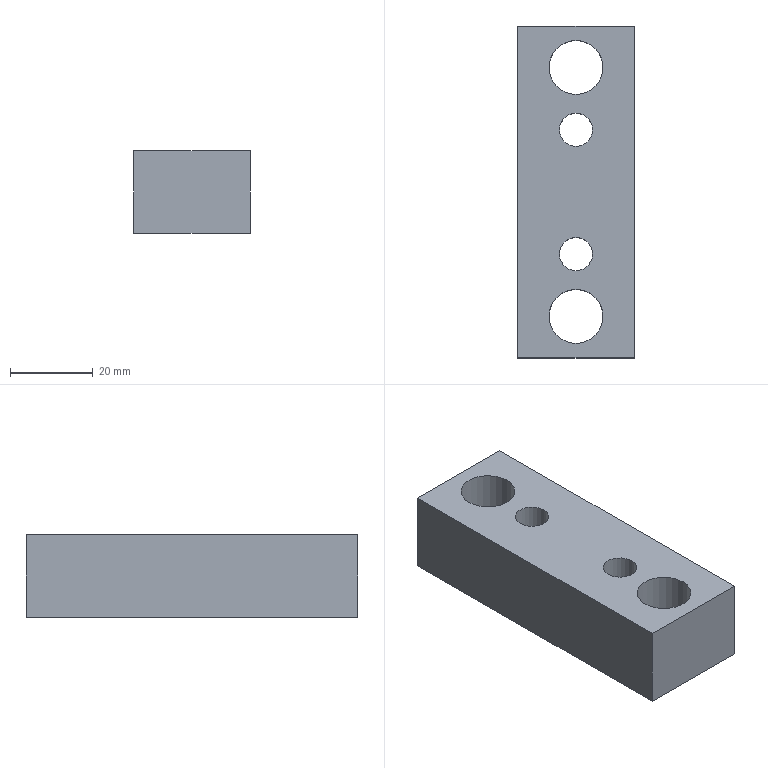Part | NX | features solid 2 | 1 solid | 10 faces | box 28 x 80 x 20 mm | volume 37480 mm3 | plane 6 | cylinder 4 | commonest cylinder face diameters 8 x2 13 x2
STEP:
#1=CARTESIAN_POINT('',(-1190.,-545.,-125.));
#2=VERTEX_POINT('',#1);
#3=CARTESIAN_POINT('',(-1190.,-625.,-125.));
#4=VERTEX_POINT('',#3);
#5=CARTESIAN_POINT('',(-1190.,-545.,-125.));
#6=DIRECTION('',(0.,-1.,0.));
#7=VECTOR('',#6,1000.);
#8=LINE('',#5,#7);
#9=EDGE_CURVE('',#2,#4,#8,.T.);
#10=ORIENTED_EDGE('',*,*,#9,.F.);
#11=CARTESIAN_POINT('',(-1190.,-545.,-105.));
#12=VERTEX_POINT('',#11);
#13=CARTESIAN_POINT('',(-1190.,-545.,-105.));
#14=DIRECTION('',(0.,0.,-1.));
#15=VECTOR('',#14,1000.);
#16=LINE('',#13,#15);
#17=EDGE_CURVE('',#12,#2,#16,.T.);
#18=ORIENTED_EDGE('',*,*,#17,.F.);
#19=CARTESIAN_POINT('',(-1190.,-625.,-105.));
#20=VERTEX_POINT('',#19);
#21=CARTESIAN_POINT('',(-1190.,-545.,-105.));
#22=DIRECTION('',(0.,-1.,0.));
#23=VECTOR('',#22,1000.);
#24=LINE('',#21,#23);
#25=EDGE_CURVE('',#12,#20,#24,.T.);
#26=ORIENTED_EDGE('',*,*,#25,.T.);
#27=CARTESIAN_POINT('',(-1190.,-625.,-105.));
#28=DIRECTION('',(0.,0.,-1.));
#29=VECTOR('',#28,1000.);
#30=LINE('',#27,#29);
#31=EDGE_CURVE('',#20,#4,#30,.T.);
#32=ORIENTED_EDGE('',*,*,#31,.T.);
#33=EDGE_LOOP('',(#10,#18,#26,#32));
#34=FACE_BOUND('',#33,.T.);
#35=CARTESIAN_POINT('',(-1190.,-545.,-105.));
#36=DIRECTION('',(1.,0.,0.));
#37=DIRECTION('',(0.,1.,0.));
#38=AXIS2_PLACEMENT_3D('',#35,#36,#37);
#39=PLANE('',#38);
#40=ADVANCED_FACE('',(#34),#39,.T.);
#41=CARTESIAN_POINT('',(-1218.,-625.,-125.));
#42=VERTEX_POINT('',#41);
#43=CARTESIAN_POINT('',(-1190.,-625.,-125.));
#44=DIRECTION('',(-1.,0.,0.));
#45=VECTOR('',#44,1000.);
#46=LINE('',#43,#45);
#47=EDGE_CURVE('',#4,#42,#46,.T.);
#48=ORIENTED_EDGE('',*,*,#47,.F.);
#49=ORIENTED_EDGE('',*,*,#31,.F.);
#50=CARTESIAN_POINT('',(-1218.,-625.,-105.));
#51=VERTEX_POINT('',#50);
#52=CARTESIAN_POINT('',(-1190.,-625.,-105.));
#53=DIRECTION('',(-1.,0.,0.));
#54=VECTOR('',#53,1000.);
#55=LINE('',#52,#54);
#56=EDGE_CURVE('',#20,#51,#55,.T.);
#57=ORIENTED_EDGE('',*,*,#56,.T.);
#58=CARTESIAN_POINT('',(-1218.,-625.,-105.));
#59=DIRECTION('',(0.,0.,-1.));
#60=VECTOR('',#59,1000.);
#61=LINE('',#58,#60);
#62=EDGE_CURVE('',#51,#42,#61,.T.);
#63=ORIENTED_EDGE('',*,*,#62,.T.);
#64=EDGE_LOOP('',(#48,#49,#57,#63));
#65=FACE_BOUND('',#64,.T.);
#66=CARTESIAN_POINT('',(-1190.,-625.,-105.));
#67=DIRECTION('',(0.,-1.,0.));
#68=DIRECTION('',(0.,0.,1.));
#69=AXIS2_PLACEMENT_3D('',#66,#67,#68);
#70=PLANE('',#69);
#71=ADVANCED_FACE('',(#65),#70,.T.);
#72=CARTESIAN_POINT('',(-1218.,-545.,-125.));
#73=VERTEX_POINT('',#72);
#74=CARTESIAN_POINT('',(-1218.,-625.,-125.));
#75=DIRECTION('',(0.,1.,0.));
#76=VECTOR('',#75,1000.);
#77=LINE('',#74,#76);
#78=EDGE_CURVE('',#42,#73,#77,.T.);
#79=ORIENTED_EDGE('',*,*,#78,.F.);
#80=ORIENTED_EDGE('',*,*,#62,.F.);
#81=CARTESIAN_POINT('',(-1218.,-545.,-105.));
#82=VERTEX_POINT('',#81);
#83=CARTESIAN_POINT('',(-1218.,-625.,-105.));
#84=DIRECTION('',(0.,1.,0.));
#85=VECTOR('',#84,1000.);
#86=LINE('',#83,#85);
#87=EDGE_CURVE('',#51,#82,#86,.T.);
#88=ORIENTED_EDGE('',*,*,#87,.T.);
#89=CARTESIAN_POINT('',(-1218.,-545.,-105.));
#90=DIRECTION('',(0.,0.,-1.));
#91=VECTOR('',#90,1000.);
#92=LINE('',#89,#91);
#93=EDGE_CURVE('',#82,#73,#92,.T.);
#94=ORIENTED_EDGE('',*,*,#93,.T.);
#95=EDGE_LOOP('',(#79,#80,#88,#94));
#96=FACE_BOUND('',#95,.T.);
#97=CARTESIAN_POINT('',(-1218.,-625.,-105.));
#98=DIRECTION('',(-1.,0.,0.));
#99=DIRECTION('',(0.,-1.,0.));
#100=AXIS2_PLACEMENT_3D('',#97,#98,#99);
#101=PLANE('',#100);
#102=ADVANCED_FACE('',(#96),#101,.T.);
#103=CARTESIAN_POINT('',(-1208.,-600.,-105.));
#104=VERTEX_POINT('',#103);
#105=CARTESIAN_POINT('',(-1204.,-600.,-105.));
#106=DIRECTION('',(0.,0.,1.));
#107=DIRECTION('',(-1.,0.,0.));
#108=AXIS2_PLACEMENT_3D('',#105,#106,#107);
#109=CIRCLE('',#108,4.);
#110=EDGE_CURVE('',#104,#104,#109,.T.);
#111=ORIENTED_EDGE('',*,*,#110,.T.);
#112=EDGE_LOOP('',(#111));
#113=FACE_BOUND('',#112,.T.);
#114=CARTESIAN_POINT('',(-1208.,-600.,-125.));
#115=VERTEX_POINT('',#114);
#116=CARTESIAN_POINT('',(-1204.,-600.,-125.));
#117=DIRECTION('',(0.,0.,1.));
#118=DIRECTION('',(-1.,0.,0.));
#119=AXIS2_PLACEMENT_3D('',#116,#117,#118);
#120=CIRCLE('',#119,4.);
#121=EDGE_CURVE('',#115,#115,#120,.T.);
#122=ORIENTED_EDGE('',*,*,#121,.F.);
#123=EDGE_LOOP('',(#122));
#124=FACE_BOUND('',#123,.T.);
#125=CARTESIAN_POINT('',(-1204.,-600.,-105.));
#126=DIRECTION('',(0.,0.,-1.));
#127=DIRECTION('',(1.,0.,0.));
#128=AXIS2_PLACEMENT_3D('',#125,#126,#127);
#129=CYLINDRICAL_SURFACE('',#128,4.);
#130=ADVANCED_FACE('',(#113,#124),#129,.F.);
#131=CARTESIAN_POINT('',(-1218.,-545.,-125.));
#132=DIRECTION('',(1.,0.,0.));
#133=VECTOR('',#132,1000.);
#134=LINE('',#131,#133);
#135=EDGE_CURVE('',#73,#2,#134,.T.);
#136=ORIENTED_EDGE('',*,*,#135,.F.);
#137=ORIENTED_EDGE('',*,*,#93,.F.);
#138=CARTESIAN_POINT('',(-1218.,-545.,-105.));
#139=DIRECTION('',(1.,0.,0.));
#140=VECTOR('',#139,1000.);
#141=LINE('',#138,#140);
#142=EDGE_CURVE('',#82,#12,#141,.T.);
#143=ORIENTED_EDGE('',*,*,#142,.T.);
#144=ORIENTED_EDGE('',*,*,#17,.T.);
#145=EDGE_LOOP('',(#136,#137,#143,#144));
#146=FACE_BOUND('',#145,.T.);
#147=CARTESIAN_POINT('',(-1218.,-545.,-105.));
#148=DIRECTION('',(0.,1.,0.));
#149=DIRECTION('',(-1.,0.,0.));
#150=AXIS2_PLACEMENT_3D('',#147,#148,#149);
#151=PLANE('',#150);
#152=ADVANCED_FACE('',(#146),#151,.T.);
#153=CARTESIAN_POINT('',(-1210.5,-615.,-105.));
#154=VERTEX_POINT('',#153);
#155=CARTESIAN_POINT('',(-1204.,-615.,-105.));
#156=DIRECTION('',(0.,0.,1.));
#157=DIRECTION('',(-1.,0.,0.));
#158=AXIS2_PLACEMENT_3D('',#155,#156,#157);
#159=CIRCLE('',#158,6.5);
#160=EDGE_CURVE('',#154,#154,#159,.T.);
#161=ORIENTED_EDGE('',*,*,#160,.T.);
#162=EDGE_LOOP('',(#161));
#163=FACE_BOUND('',#162,.T.);
#164=CARTESIAN_POINT('',(-1210.5,-615.,-125.));
#165=VERTEX_POINT('',#164);
#166=CARTESIAN_POINT('',(-1204.,-615.,-125.));
#167=DIRECTION('',(0.,0.,1.));
#168=DIRECTION('',(-1.,0.,0.));
#169=AXIS2_PLACEMENT_3D('',#166,#167,#168);
#170=CIRCLE('',#169,6.5);
#171=EDGE_CURVE('',#165,#165,#170,.T.);
#172=ORIENTED_EDGE('',*,*,#171,.F.);
#173=EDGE_LOOP('',(#172));
#174=FACE_BOUND('',#173,.T.);
#175=CARTESIAN_POINT('',(-1204.,-615.,-105.));
#176=DIRECTION('',(0.,0.,-1.));
#177=DIRECTION('',(1.,0.,0.));
#178=AXIS2_PLACEMENT_3D('',#175,#176,#177);
#179=CYLINDRICAL_SURFACE('',#178,6.5);
#180=ADVANCED_FACE('',(#163,#174),#179,.F.);
#181=CARTESIAN_POINT('',(-1208.,-570.,-105.));
#182=VERTEX_POINT('',#181);
#183=CARTESIAN_POINT('',(-1204.,-570.,-105.));
#184=DIRECTION('',(0.,0.,1.));
#185=DIRECTION('',(-1.,0.,0.));
#186=AXIS2_PLACEMENT_3D('',#183,#184,#185);
#187=CIRCLE('',#186,4.);
#188=EDGE_CURVE('',#182,#182,#187,.T.);
#189=ORIENTED_EDGE('',*,*,#188,.T.);
#190=EDGE_LOOP('',(#189));
#191=FACE_BOUND('',#190,.T.);
#192=CARTESIAN_POINT('',(-1208.,-570.,-125.));
#193=VERTEX_POINT('',#192);
#194=CARTESIAN_POINT('',(-1204.,-570.,-125.));
#195=DIRECTION('',(0.,0.,1.));
#196=DIRECTION('',(-1.,0.,0.));
#197=AXIS2_PLACEMENT_3D('',#194,#195,#196);
#198=CIRCLE('',#197,4.);
#199=EDGE_CURVE('',#193,#193,#198,.T.);
#200=ORIENTED_EDGE('',*,*,#199,.F.);
#201=EDGE_LOOP('',(#200));
#202=FACE_BOUND('',#201,.T.);
#203=CARTESIAN_POINT('',(-1204.,-570.,-105.));
#204=DIRECTION('',(0.,0.,-1.));
#205=DIRECTION('',(1.,0.,0.));
#206=AXIS2_PLACEMENT_3D('',#203,#204,#205);
#207=CYLINDRICAL_SURFACE('',#206,4.);
#208=ADVANCED_FACE('',(#191,#202),#207,.F.);
#209=CARTESIAN_POINT('',(-1210.5,-555.,-105.));
#210=VERTEX_POINT('',#209);
#211=CARTESIAN_POINT('',(-1204.,-555.,-105.));
#212=DIRECTION('',(0.,0.,1.));
#213=DIRECTION('',(-1.,0.,0.));
#214=AXIS2_PLACEMENT_3D('',#211,#212,#213);
#215=CIRCLE('',#214,6.5);
#216=EDGE_CURVE('',#210,#210,#215,.T.);
#217=ORIENTED_EDGE('',*,*,#216,.T.);
#218=EDGE_LOOP('',(#217));
#219=FACE_BOUND('',#218,.T.);
#220=CARTESIAN_POINT('',(-1210.5,-555.,-125.));
#221=VERTEX_POINT('',#220);
#222=CARTESIAN_POINT('',(-1204.,-555.,-125.));
#223=DIRECTION('',(0.,0.,1.));
#224=DIRECTION('',(-1.,0.,0.));
#225=AXIS2_PLACEMENT_3D('',#222,#223,#224);
#226=CIRCLE('',#225,6.5);
#227=EDGE_CURVE('',#221,#221,#226,.T.);
#228=ORIENTED_EDGE('',*,*,#227,.F.);
#229=EDGE_LOOP('',(#228));
#230=FACE_BOUND('',#229,.T.);
#231=CARTESIAN_POINT('',(-1204.,-555.,-105.));
#232=DIRECTION('',(0.,0.,-1.));
#233=DIRECTION('',(1.,0.,0.));
#234=AXIS2_PLACEMENT_3D('',#231,#232,#233);
#235=CYLINDRICAL_SURFACE('',#234,6.5);
#236=ADVANCED_FACE('',(#219,#230),#235,.F.);
#237=ORIENTED_EDGE('',*,*,#188,.F.);
#238=EDGE_LOOP('',(#237));
#239=FACE_BOUND('',#238,.T.);
#240=ORIENTED_EDGE('',*,*,#160,.F.);
#241=EDGE_LOOP('',(#240));
#242=FACE_BOUND('',#241,.T.);
#243=ORIENTED_EDGE('',*,*,#25,.F.);
#244=ORIENTED_EDGE('',*,*,#142,.F.);
#245=ORIENTED_EDGE('',*,*,#87,.F.);
#246=ORIENTED_EDGE('',*,*,#56,.F.);
#247=EDGE_LOOP('',(#243,#244,#245,#246));
#248=FACE_BOUND('',#247,.T.);
#249=ORIENTED_EDGE('',*,*,#110,.F.);
#250=EDGE_LOOP('',(#249));
#251=FACE_BOUND('',#250,.T.);
#252=ORIENTED_EDGE('',*,*,#216,.F.);
#253=EDGE_LOOP('',(#252));
#254=FACE_BOUND('',#253,.T.);
#255=CARTESIAN_POINT('',(-1190.,-545.,-105.));
#256=DIRECTION('',(0.,0.,1.));
#257=DIRECTION('',(-1.,0.,0.));
#258=AXIS2_PLACEMENT_3D('',#255,#256,#257);
#259=PLANE('',#258);
#260=ADVANCED_FACE('',(#239,#242,#248,#251,#254),#259,.T.);
#261=ORIENTED_EDGE('',*,*,#199,.T.);
#262=EDGE_LOOP('',(#261));
#263=FACE_BOUND('',#262,.T.);
#264=ORIENTED_EDGE('',*,*,#171,.T.);
#265=EDGE_LOOP('',(#264));
#266=FACE_BOUND('',#265,.T.);
#267=ORIENTED_EDGE('',*,*,#9,.T.);
#268=ORIENTED_EDGE('',*,*,#47,.T.);
#269=ORIENTED_EDGE('',*,*,#78,.T.);
#270=ORIENTED_EDGE('',*,*,#135,.T.);
#271=EDGE_LOOP('',(#267,#268,#269,#270));
#272=FACE_BOUND('',#271,.T.);
#273=ORIENTED_EDGE('',*,*,#121,.T.);
#274=EDGE_LOOP('',(#273));
#275=FACE_BOUND('',#274,.T.);
#276=ORIENTED_EDGE('',*,*,#227,.T.);
#277=EDGE_LOOP('',(#276));
#278=FACE_BOUND('',#277,.T.);
#279=CARTESIAN_POINT('',(-1190.,-545.,-125.));
#280=DIRECTION('',(0.,0.,1.));
#281=DIRECTION('',(-1.,0.,0.));
#282=AXIS2_PLACEMENT_3D('',#279,#280,#281);
#283=PLANE('',#282);
#284=ADVANCED_FACE('',(#263,#266,#272,#275,#278),#283,.F.);
#285=CLOSED_SHELL('',(#40,#71,#102,#130,#152,#180,#208,#236,#260,#284));
#286=MANIFOLD_SOLID_BREP('',#285);
#287=(LENGTH_UNIT()NAMED_UNIT(*)SI_UNIT(.MILLI.,.METRE.));
#288=UNCERTAINTY_MEASURE_WITH_UNIT(LENGTH_MEASURE(0.00001),#287,'','');
#289=(NAMED_UNIT(*)PLANE_ANGLE_UNIT()SI_UNIT($,.RADIAN.));
#290=(NAMED_UNIT(*)SI_UNIT($,.STERADIAN.)SOLID_ANGLE_UNIT());
#291=(GEOMETRIC_REPRESENTATION_CONTEXT(3)GLOBAL_UNCERTAINTY_ASSIGNED_CONTEXT((#288))GLOBAL_UNIT_ASSIGNED_CONTEXT((#287,#289,#290))REPRESENTATION_CONTEXT('',''));
#292=ADVANCED_BREP_SHAPE_REPRESENTATION('',(#286),#291);